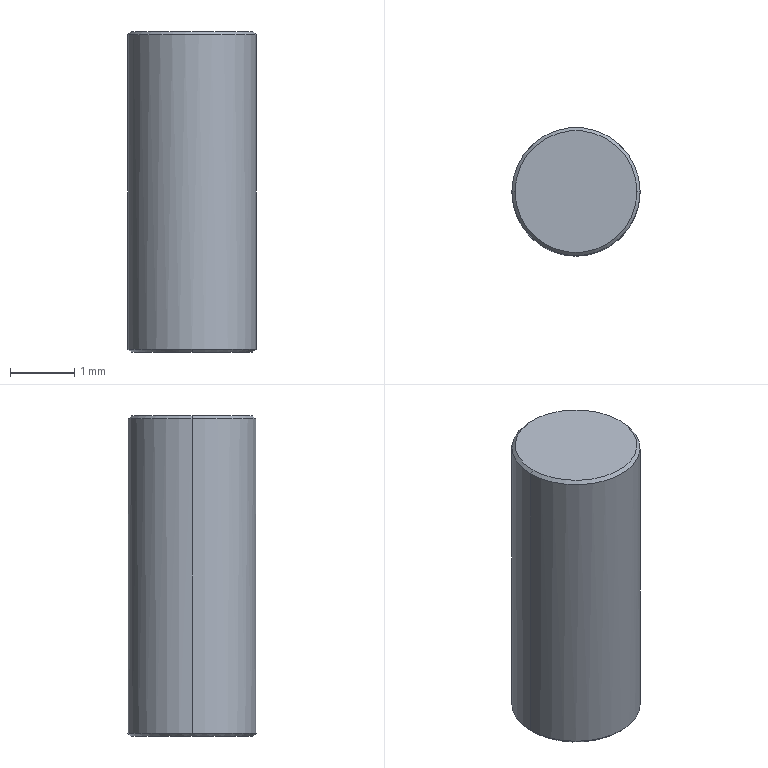Part | SolidWorks | features BaseBody 1 | 1 solid | 8 faces | box 2 x 2 x 5 mm | volume 15.693 mm3 | cone 4 | cylinder 2 | plane 2 | commonest cylinder face diameters 2 x2
STEP:
#1=CARTESIAN_POINT('',(-22.185,10.496,0.05));
#2=VERTEX_POINT('',#1);
#3=CARTESIAN_POINT('',(-23.185,9.496,0.05));
#4=VERTEX_POINT('',#3);
#5=CARTESIAN_POINT('',(-22.185,9.496,0.05));
#6=DIRECTION('',(0.,0.,1.));
#7=DIRECTION('',(1.,0.,0.));
#8=AXIS2_PLACEMENT_3D('',#5,#6,#7);
#9=CIRCLE('',#8,1.);
#10=EDGE_CURVE('',#2,#4,#9,.T.);
#11=ORIENTED_EDGE('',*,*,#10,.T.);
#12=CARTESIAN_POINT('',(-23.185,9.496,4.95));
#13=VERTEX_POINT('',#12);
#14=CARTESIAN_POINT('',(-23.185,9.496,0.));
#15=DIRECTION('',(0.,0.,1.));
#16=VECTOR('',#15,1000.);
#17=LINE('',#14,#16);
#18=EDGE_CURVE('',#4,#13,#17,.T.);
#19=ORIENTED_EDGE('',*,*,#18,.T.);
#20=CARTESIAN_POINT('',(-21.185,9.496,4.95));
#21=VERTEX_POINT('',#20);
#22=CARTESIAN_POINT('',(-22.185,9.496,4.95));
#23=DIRECTION('',(0.,0.,-1.));
#24=DIRECTION('',(1.,0.,0.));
#25=AXIS2_PLACEMENT_3D('',#22,#23,#24);
#26=CIRCLE('',#25,1.);
#27=EDGE_CURVE('',#13,#21,#26,.T.);
#28=ORIENTED_EDGE('',*,*,#27,.T.);
#29=CARTESIAN_POINT('',(-21.185,9.496,0.05));
#30=VERTEX_POINT('',#29);
#31=CARTESIAN_POINT('',(-21.185,9.496,0.));
#32=DIRECTION('',(0.,0.,1.));
#33=VECTOR('',#32,1000.);
#34=LINE('',#31,#33);
#35=EDGE_CURVE('',#30,#21,#34,.T.);
#36=ORIENTED_EDGE('',*,*,#35,.F.);
#37=CARTESIAN_POINT('',(-22.185,9.496,0.05));
#38=DIRECTION('',(0.,0.,1.));
#39=DIRECTION('',(1.,0.,0.));
#40=AXIS2_PLACEMENT_3D('',#37,#38,#39);
#41=CIRCLE('',#40,1.);
#42=EDGE_CURVE('',#30,#2,#41,.T.);
#43=ORIENTED_EDGE('',*,*,#42,.T.);
#44=EDGE_LOOP('',(#11,#19,#28,#36,#43));
#45=FACE_OUTER_BOUND('',#44,.T.);
#46=CARTESIAN_POINT('',(-22.185,9.496,0.));
#47=DIRECTION('',(0.,0.,1.));
#48=DIRECTION('',(1.,0.,0.));
#49=AXIS2_PLACEMENT_3D('',#46,#47,#48);
#50=CYLINDRICAL_SURFACE('',#49,1.);
#51=ADVANCED_FACE('',(#45),#50,.T.);
#52=CARTESIAN_POINT('',(-22.185,8.546,0.));
#53=VERTEX_POINT('',#52);
#54=CARTESIAN_POINT('',(-22.185,10.446,0.));
#55=VERTEX_POINT('',#54);
#56=CARTESIAN_POINT('',(-22.185,9.496,0.));
#57=DIRECTION('',(0.,0.,1.));
#58=DIRECTION('',(0.,-1.,0.));
#59=AXIS2_PLACEMENT_3D('',#56,#57,#58);
#60=CIRCLE('',#59,0.95);
#61=EDGE_CURVE('',#53,#55,#60,.T.);
#62=ORIENTED_EDGE('',*,*,#61,.T.);
#63=CARTESIAN_POINT('',(-22.185,10.496,0.05));
#64=DIRECTION('',(0.,0.7071,0.7071));
#65=VECTOR('',#64,1000.);
#66=LINE('',#63,#65);
#67=EDGE_CURVE('',#55,#2,#66,.T.);
#68=ORIENTED_EDGE('',*,*,#67,.T.);
#69=ORIENTED_EDGE('',*,*,#42,.F.);
#70=CARTESIAN_POINT('',(-22.185,8.496,0.05));
#71=VERTEX_POINT('',#70);
#72=CARTESIAN_POINT('',(-22.185,9.496,0.05));
#73=DIRECTION('',(0.,0.,1.));
#74=DIRECTION('',(1.,0.,0.));
#75=AXIS2_PLACEMENT_3D('',#72,#73,#74);
#76=CIRCLE('',#75,1.);
#77=EDGE_CURVE('',#71,#30,#76,.T.);
#78=ORIENTED_EDGE('',*,*,#77,.F.);
#79=CARTESIAN_POINT('',(-22.185,8.496,0.05));
#80=DIRECTION('',(0.,-0.7071,0.7071));
#81=VECTOR('',#80,1000.);
#82=LINE('',#79,#81);
#83=EDGE_CURVE('',#53,#71,#82,.T.);
#84=ORIENTED_EDGE('',*,*,#83,.F.);
#85=EDGE_LOOP('',(#62,#68,#69,#78,#84));
#86=FACE_OUTER_BOUND('',#85,.T.);
#87=CARTESIAN_POINT('',(-22.185,9.496,0.05));
#88=DIRECTION('',(0.,0.,1.));
#89=DIRECTION('',(0.,-1.,0.));
#90=AXIS2_PLACEMENT_3D('',#87,#88,#89);
#91=CONICAL_SURFACE('',#90,1.,0.7854);
#92=ADVANCED_FACE('',(#86),#91,.T.);
#93=CARTESIAN_POINT('',(-23.135,9.496,5.));
#94=VERTEX_POINT('',#93);
#95=CARTESIAN_POINT('',(-21.235,9.496,5.));
#96=VERTEX_POINT('',#95);
#97=CARTESIAN_POINT('',(-22.185,9.496,5.));
#98=DIRECTION('',(0.,0.,-1.));
#99=DIRECTION('',(-1.,0.,0.));
#100=AXIS2_PLACEMENT_3D('',#97,#98,#99);
#101=CIRCLE('',#100,0.95);
#102=EDGE_CURVE('',#94,#96,#101,.T.);
#103=ORIENTED_EDGE('',*,*,#102,.T.);
#104=CARTESIAN_POINT('',(-21.185,9.496,4.95));
#105=DIRECTION('',(0.7071,0.,-0.7071));
#106=VECTOR('',#105,1000.);
#107=LINE('',#104,#106);
#108=EDGE_CURVE('',#96,#21,#107,.T.);
#109=ORIENTED_EDGE('',*,*,#108,.T.);
#110=ORIENTED_EDGE('',*,*,#27,.F.);
#111=CARTESIAN_POINT('',(-23.185,9.496,4.95));
#112=DIRECTION('',(-0.7071,0.,-0.7071));
#113=VECTOR('',#112,1000.);
#114=LINE('',#111,#113);
#115=EDGE_CURVE('',#94,#13,#114,.T.);
#116=ORIENTED_EDGE('',*,*,#115,.F.);
#117=EDGE_LOOP('',(#103,#109,#110,#116));
#118=FACE_OUTER_BOUND('',#117,.T.);
#119=CARTESIAN_POINT('',(-22.185,9.496,4.95));
#120=DIRECTION('',(0.,0.,-1.));
#121=DIRECTION('',(-1.,0.,0.));
#122=AXIS2_PLACEMENT_3D('',#119,#120,#121);
#123=CONICAL_SURFACE('',#122,1.,0.7854);
#124=ADVANCED_FACE('',(#118),#123,.T.);
#125=ORIENTED_EDGE('',*,*,#18,.F.);
#126=CARTESIAN_POINT('',(-22.185,9.496,0.05));
#127=DIRECTION('',(0.,0.,1.));
#128=DIRECTION('',(1.,0.,0.));
#129=AXIS2_PLACEMENT_3D('',#126,#127,#128);
#130=CIRCLE('',#129,1.);
#131=EDGE_CURVE('',#4,#71,#130,.T.);
#132=ORIENTED_EDGE('',*,*,#131,.T.);
#133=ORIENTED_EDGE('',*,*,#77,.T.);
#134=ORIENTED_EDGE('',*,*,#35,.T.);
#135=CARTESIAN_POINT('',(-22.185,9.496,4.95));
#136=DIRECTION('',(0.,0.,-1.));
#137=DIRECTION('',(1.,0.,0.));
#138=AXIS2_PLACEMENT_3D('',#135,#136,#137);
#139=CIRCLE('',#138,1.);
#140=EDGE_CURVE('',#21,#13,#139,.T.);
#141=ORIENTED_EDGE('',*,*,#140,.T.);
#142=EDGE_LOOP('',(#125,#132,#133,#134,#141));
#143=FACE_OUTER_BOUND('',#142,.T.);
#144=CARTESIAN_POINT('',(-22.185,9.496,0.));
#145=DIRECTION('',(0.,0.,1.));
#146=DIRECTION('',(1.,0.,0.));
#147=AXIS2_PLACEMENT_3D('',#144,#145,#146);
#148=CYLINDRICAL_SURFACE('',#147,1.);
#149=ADVANCED_FACE('',(#143),#148,.T.);
#150=ORIENTED_EDGE('',*,*,#67,.F.);
#151=CARTESIAN_POINT('',(-22.185,9.496,0.));
#152=DIRECTION('',(0.,0.,1.));
#153=DIRECTION('',(0.,-1.,0.));
#154=AXIS2_PLACEMENT_3D('',#151,#152,#153);
#155=CIRCLE('',#154,0.95);
#156=EDGE_CURVE('',#55,#53,#155,.T.);
#157=ORIENTED_EDGE('',*,*,#156,.T.);
#158=ORIENTED_EDGE('',*,*,#83,.T.);
#159=ORIENTED_EDGE('',*,*,#131,.F.);
#160=ORIENTED_EDGE('',*,*,#10,.F.);
#161=EDGE_LOOP('',(#150,#157,#158,#159,#160));
#162=FACE_OUTER_BOUND('',#161,.T.);
#163=CARTESIAN_POINT('',(-22.185,9.496,0.05));
#164=DIRECTION('',(0.,0.,1.));
#165=DIRECTION('',(0.,-1.,0.));
#166=AXIS2_PLACEMENT_3D('',#163,#164,#165);
#167=CONICAL_SURFACE('',#166,1.,0.7854);
#168=ADVANCED_FACE('',(#162),#167,.T.);
#169=ORIENTED_EDGE('',*,*,#108,.F.);
#170=CARTESIAN_POINT('',(-22.185,9.496,5.));
#171=DIRECTION('',(0.,0.,-1.));
#172=DIRECTION('',(-1.,0.,0.));
#173=AXIS2_PLACEMENT_3D('',#170,#171,#172);
#174=CIRCLE('',#173,0.95);
#175=EDGE_CURVE('',#96,#94,#174,.T.);
#176=ORIENTED_EDGE('',*,*,#175,.T.);
#177=ORIENTED_EDGE('',*,*,#115,.T.);
#178=ORIENTED_EDGE('',*,*,#140,.F.);
#179=EDGE_LOOP('',(#169,#176,#177,#178));
#180=FACE_OUTER_BOUND('',#179,.T.);
#181=CARTESIAN_POINT('',(-22.185,9.496,4.95));
#182=DIRECTION('',(0.,0.,-1.));
#183=DIRECTION('',(-1.,0.,0.));
#184=AXIS2_PLACEMENT_3D('',#181,#182,#183);
#185=CONICAL_SURFACE('',#184,1.,0.7854);
#186=ADVANCED_FACE('',(#180),#185,.T.);
#187=ORIENTED_EDGE('',*,*,#61,.F.);
#188=ORIENTED_EDGE('',*,*,#156,.F.);
#189=EDGE_LOOP('',(#187,#188));
#190=FACE_OUTER_BOUND('',#189,.T.);
#191=CARTESIAN_POINT('',(-22.185,9.496,0.));
#192=DIRECTION('',(0.,0.,-1.));
#193=DIRECTION('',(-1.,0.,0.));
#194=AXIS2_PLACEMENT_3D('',#191,#192,#193);
#195=PLANE('',#194);
#196=ADVANCED_FACE('',(#190),#195,.T.);
#197=ORIENTED_EDGE('',*,*,#102,.F.);
#198=ORIENTED_EDGE('',*,*,#175,.F.);
#199=EDGE_LOOP('',(#197,#198));
#200=FACE_OUTER_BOUND('',#199,.T.);
#201=CARTESIAN_POINT('',(-22.185,9.496,5.));
#202=DIRECTION('',(0.,0.,-1.));
#203=DIRECTION('',(-1.,0.,0.));
#204=AXIS2_PLACEMENT_3D('',#201,#202,#203);
#205=PLANE('',#204);
#206=ADVANCED_FACE('',(#200),#205,.F.);
#207=CLOSED_SHELL('',(#51,#92,#124,#149,#168,#186,#196,#206));
#208=MANIFOLD_SOLID_BREP('',#207);
#209=CARTESIAN_POINT('',(0.,0.,0.));
#210=DIRECTION('',(0.,0.,1.));
#211=DIRECTION('',(1.,0.,0.));
#212=AXIS2_PLACEMENT_3D('',#209,#210,#211);
#213=(LENGTH_UNIT()NAMED_UNIT(*)SI_UNIT(.MILLI.,.METRE.));
#214=UNCERTAINTY_MEASURE_WITH_UNIT(LENGTH_MEASURE(0.00001),#213,'','');
#215=(NAMED_UNIT(*)PLANE_ANGLE_UNIT()SI_UNIT($,.RADIAN.));
#216=(NAMED_UNIT(*)SI_UNIT($,.STERADIAN.)SOLID_ANGLE_UNIT());
#217=(GEOMETRIC_REPRESENTATION_CONTEXT(3)GLOBAL_UNCERTAINTY_ASSIGNED_CONTEXT((#214))GLOBAL_UNIT_ASSIGNED_CONTEXT((#213,#215,#216))REPRESENTATION_CONTEXT('',''));
#218=ADVANCED_BREP_SHAPE_REPRESENTATION('',(#208,#212),#217);